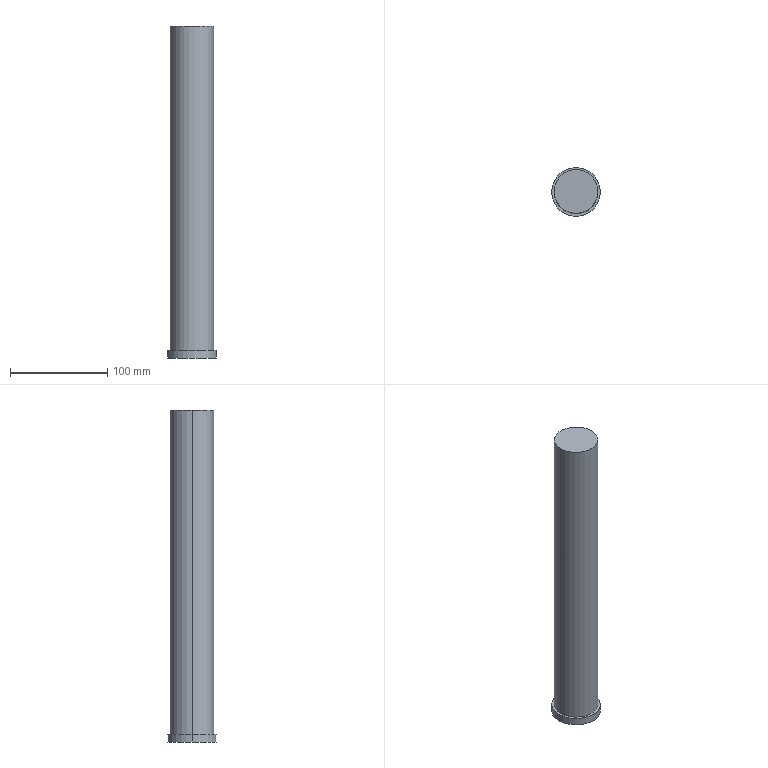Part | SolidWorks | features BaseBody 1 | 1 solid | 7 faces | box 50 x 50 x 341 mm | volume 545322 mm3 | cylinder 4 | plane 3 | commonest cylinder face diameters 45 x2 50 x2
STEP:
#1=CARTESIAN_POINT('',(-370.,180.,-340.5));
#2=VERTEX_POINT('',#1);
#3=CARTESIAN_POINT('',(-320.,180.,-340.5));
#4=VERTEX_POINT('',#3);
#5=CARTESIAN_POINT('',(-345.,180.,-340.5));
#6=DIRECTION('',(0.,0.,1.));
#7=DIRECTION('',(-1.,0.,0.));
#8=AXIS2_PLACEMENT_3D('',#5,#6,#7);
#9=CIRCLE('',#8,25.);
#10=EDGE_CURVE('',#2,#4,#9,.T.);
#11=ORIENTED_EDGE('',*,*,#10,.T.);
#12=CARTESIAN_POINT('',(-320.,180.,-332.5));
#13=VERTEX_POINT('',#12);
#14=CARTESIAN_POINT('',(-320.,180.,-340.5));
#15=DIRECTION('',(0.,0.,1.));
#16=VECTOR('',#15,1000.);
#17=LINE('',#14,#16);
#18=EDGE_CURVE('',#4,#13,#17,.T.);
#19=ORIENTED_EDGE('',*,*,#18,.T.);
#20=CARTESIAN_POINT('',(-370.,180.,-332.5));
#21=VERTEX_POINT('',#20);
#22=CARTESIAN_POINT('',(-345.,180.,-332.5));
#23=DIRECTION('',(0.,0.,1.));
#24=DIRECTION('',(-1.,0.,0.));
#25=AXIS2_PLACEMENT_3D('',#22,#23,#24);
#26=CIRCLE('',#25,25.);
#27=EDGE_CURVE('',#21,#13,#26,.T.);
#28=ORIENTED_EDGE('',*,*,#27,.F.);
#29=CARTESIAN_POINT('',(-370.,180.,-340.5));
#30=DIRECTION('',(0.,0.,1.));
#31=VECTOR('',#30,1000.);
#32=LINE('',#29,#31);
#33=EDGE_CURVE('',#2,#21,#32,.T.);
#34=ORIENTED_EDGE('',*,*,#33,.F.);
#35=EDGE_LOOP('',(#11,#19,#28,#34));
#36=FACE_OUTER_BOUND('',#35,.T.);
#37=CARTESIAN_POINT('',(-345.,180.,-340.5));
#38=DIRECTION('',(0.,0.,1.));
#39=DIRECTION('',(-1.,0.,0.));
#40=AXIS2_PLACEMENT_3D('',#37,#38,#39);
#41=CYLINDRICAL_SURFACE('',#40,25.);
#42=ADVANCED_FACE('',(#36),#41,.T.);
#43=CARTESIAN_POINT('',(-322.5,180.,0.5));
#44=VERTEX_POINT('',#43);
#45=CARTESIAN_POINT('',(-367.5,180.,0.5));
#46=VERTEX_POINT('',#45);
#47=CARTESIAN_POINT('',(-345.,180.,0.5));
#48=DIRECTION('',(0.,0.,-1.));
#49=DIRECTION('',(-1.,0.,0.));
#50=AXIS2_PLACEMENT_3D('',#47,#48,#49);
#51=CIRCLE('',#50,22.5);
#52=EDGE_CURVE('',#44,#46,#51,.T.);
#53=ORIENTED_EDGE('',*,*,#52,.T.);
#54=CARTESIAN_POINT('',(-367.5,180.,-332.5));
#55=VERTEX_POINT('',#54);
#56=CARTESIAN_POINT('',(-367.5,180.,0.5));
#57=DIRECTION('',(0.,0.,-1.));
#58=VECTOR('',#57,1000.);
#59=LINE('',#56,#58);
#60=EDGE_CURVE('',#46,#55,#59,.T.);
#61=ORIENTED_EDGE('',*,*,#60,.T.);
#62=CARTESIAN_POINT('',(-322.5,180.,-332.5));
#63=VERTEX_POINT('',#62);
#64=CARTESIAN_POINT('',(-345.,180.,-332.5));
#65=DIRECTION('',(0.,0.,1.));
#66=DIRECTION('',(-1.,0.,0.));
#67=AXIS2_PLACEMENT_3D('',#64,#65,#66);
#68=CIRCLE('',#67,22.5);
#69=EDGE_CURVE('',#55,#63,#68,.T.);
#70=ORIENTED_EDGE('',*,*,#69,.T.);
#71=CARTESIAN_POINT('',(-322.5,180.,0.5));
#72=DIRECTION('',(0.,0.,-1.));
#73=VECTOR('',#72,1000.);
#74=LINE('',#71,#73);
#75=EDGE_CURVE('',#44,#63,#74,.T.);
#76=ORIENTED_EDGE('',*,*,#75,.F.);
#77=EDGE_LOOP('',(#53,#61,#70,#76));
#78=FACE_OUTER_BOUND('',#77,.T.);
#79=CARTESIAN_POINT('',(-345.,180.,0.5));
#80=DIRECTION('',(0.,0.,-1.));
#81=DIRECTION('',(1.,0.,0.));
#82=AXIS2_PLACEMENT_3D('',#79,#80,#81);
#83=CYLINDRICAL_SURFACE('',#82,22.5);
#84=ADVANCED_FACE('',(#78),#83,.T.);
#85=ORIENTED_EDGE('',*,*,#60,.F.);
#86=CARTESIAN_POINT('',(-345.,180.,0.5));
#87=DIRECTION('',(0.,0.,-1.));
#88=DIRECTION('',(-1.,0.,0.));
#89=AXIS2_PLACEMENT_3D('',#86,#87,#88);
#90=CIRCLE('',#89,22.5);
#91=EDGE_CURVE('',#46,#44,#90,.T.);
#92=ORIENTED_EDGE('',*,*,#91,.T.);
#93=ORIENTED_EDGE('',*,*,#75,.T.);
#94=CARTESIAN_POINT('',(-345.,180.,-332.5));
#95=DIRECTION('',(0.,0.,1.));
#96=DIRECTION('',(-1.,0.,0.));
#97=AXIS2_PLACEMENT_3D('',#94,#95,#96);
#98=CIRCLE('',#97,22.5);
#99=EDGE_CURVE('',#63,#55,#98,.T.);
#100=ORIENTED_EDGE('',*,*,#99,.T.);
#101=EDGE_LOOP('',(#85,#92,#93,#100));
#102=FACE_OUTER_BOUND('',#101,.T.);
#103=CARTESIAN_POINT('',(-345.,180.,0.5));
#104=DIRECTION('',(0.,0.,-1.));
#105=DIRECTION('',(1.,0.,0.));
#106=AXIS2_PLACEMENT_3D('',#103,#104,#105);
#107=CYLINDRICAL_SURFACE('',#106,22.5);
#108=ADVANCED_FACE('',(#102),#107,.T.);
#109=ORIENTED_EDGE('',*,*,#52,.F.);
#110=ORIENTED_EDGE('',*,*,#91,.F.);
#111=EDGE_LOOP('',(#109,#110));
#112=FACE_OUTER_BOUND('',#111,.T.);
#113=CARTESIAN_POINT('',(-345.,180.,0.5));
#114=DIRECTION('',(0.,0.,1.));
#115=DIRECTION('',(-1.,0.,0.));
#116=AXIS2_PLACEMENT_3D('',#113,#114,#115);
#117=PLANE('',#116);
#118=ADVANCED_FACE('',(#112),#117,.T.);
#119=ORIENTED_EDGE('',*,*,#27,.T.);
#120=CARTESIAN_POINT('',(-345.,180.,-332.5));
#121=DIRECTION('',(0.,0.,1.));
#122=DIRECTION('',(-1.,0.,0.));
#123=AXIS2_PLACEMENT_3D('',#120,#121,#122);
#124=CIRCLE('',#123,25.);
#125=EDGE_CURVE('',#13,#21,#124,.T.);
#126=ORIENTED_EDGE('',*,*,#125,.T.);
#127=EDGE_LOOP('',(#119,#126));
#128=FACE_OUTER_BOUND('',#127,.T.);
#129=ORIENTED_EDGE('',*,*,#99,.F.);
#130=ORIENTED_EDGE('',*,*,#69,.F.);
#131=EDGE_LOOP('',(#129,#130));
#132=FACE_BOUND('',#131,.T.);
#133=CARTESIAN_POINT('',(-345.,180.,-332.5));
#134=DIRECTION('',(0.,0.,1.));
#135=DIRECTION('',(-1.,0.,0.));
#136=AXIS2_PLACEMENT_3D('',#133,#134,#135);
#137=PLANE('',#136);
#138=ADVANCED_FACE('',(#128,#132),#137,.T.);
#139=ORIENTED_EDGE('',*,*,#18,.F.);
#140=CARTESIAN_POINT('',(-345.,180.,-340.5));
#141=DIRECTION('',(0.,0.,1.));
#142=DIRECTION('',(-1.,0.,0.));
#143=AXIS2_PLACEMENT_3D('',#140,#141,#142);
#144=CIRCLE('',#143,25.);
#145=EDGE_CURVE('',#4,#2,#144,.T.);
#146=ORIENTED_EDGE('',*,*,#145,.T.);
#147=ORIENTED_EDGE('',*,*,#33,.T.);
#148=ORIENTED_EDGE('',*,*,#125,.F.);
#149=EDGE_LOOP('',(#139,#146,#147,#148));
#150=FACE_OUTER_BOUND('',#149,.T.);
#151=CARTESIAN_POINT('',(-345.,180.,-340.5));
#152=DIRECTION('',(0.,0.,1.));
#153=DIRECTION('',(-1.,0.,0.));
#154=AXIS2_PLACEMENT_3D('',#151,#152,#153);
#155=CYLINDRICAL_SURFACE('',#154,25.);
#156=ADVANCED_FACE('',(#150),#155,.T.);
#157=ORIENTED_EDGE('',*,*,#10,.F.);
#158=ORIENTED_EDGE('',*,*,#145,.F.);
#159=EDGE_LOOP('',(#157,#158));
#160=FACE_OUTER_BOUND('',#159,.T.);
#161=CARTESIAN_POINT('',(-345.,180.,-340.5));
#162=DIRECTION('',(0.,0.,1.));
#163=DIRECTION('',(-1.,0.,0.));
#164=AXIS2_PLACEMENT_3D('',#161,#162,#163);
#165=PLANE('',#164);
#166=ADVANCED_FACE('',(#160),#165,.F.);
#167=CLOSED_SHELL('',(#42,#84,#108,#118,#138,#156,#166));
#168=MANIFOLD_SOLID_BREP('',#167);
#169=CARTESIAN_POINT('',(0.,0.,0.));
#170=DIRECTION('',(0.,0.,1.));
#171=DIRECTION('',(1.,0.,0.));
#172=AXIS2_PLACEMENT_3D('',#169,#170,#171);
#173=(LENGTH_UNIT()NAMED_UNIT(*)SI_UNIT(.MILLI.,.METRE.));
#174=UNCERTAINTY_MEASURE_WITH_UNIT(LENGTH_MEASURE(0.00001),#173,'','');
#175=(NAMED_UNIT(*)PLANE_ANGLE_UNIT()SI_UNIT($,.RADIAN.));
#176=(NAMED_UNIT(*)SI_UNIT($,.STERADIAN.)SOLID_ANGLE_UNIT());
#177=(GEOMETRIC_REPRESENTATION_CONTEXT(3)GLOBAL_UNCERTAINTY_ASSIGNED_CONTEXT((#174))GLOBAL_UNIT_ASSIGNED_CONTEXT((#173,#175,#176))REPRESENTATION_CONTEXT('',''));
#178=ADVANCED_BREP_SHAPE_REPRESENTATION('',(#168,#172),#177);